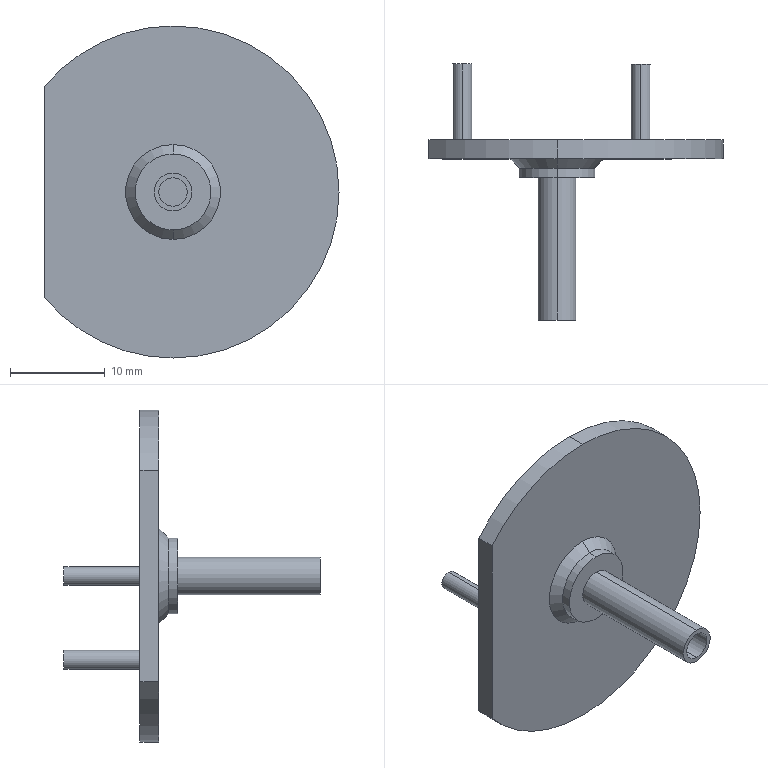Part | SolidWorks | features ICE 6, Chamfer 1, Extrusion 1 | 1 solid | 26 faces | box 31 x 27 x 35 mm | volume 2012 mm3 | cylinder 15 | plane 9 | cone 2 | commonest cylinder face diameters 2 x4 4 x4 35 x3 3 x2 8 x2
STEP:
#1=CARTESIAN_POINT('',(0.,-1.,-2.));
#2=VERTEX_POINT('',#1);
#3=CARTESIAN_POINT('',(0.,-1.,2.));
#4=VERTEX_POINT('',#3);
#5=CARTESIAN_POINT('',(0.,-1.,0.));
#6=DIRECTION('',(0.,1.,0.));
#7=DIRECTION('',(0.,0.,1.));
#8=AXIS2_PLACEMENT_3D('',#5,#6,#7);
#9=CIRCLE('',#8,2.);
#10=EDGE_CURVE('',#2,#4,#9,.T.);
#11=ORIENTED_EDGE('',*,*,#10,.F.);
#12=CARTESIAN_POINT('',(0.,2.,-2.));
#13=VERTEX_POINT('',#12);
#14=CARTESIAN_POINT('',(0.,-1.,-2.));
#15=DIRECTION('',(0.,1.,0.));
#16=VECTOR('',#15,1000.);
#17=LINE('',#14,#16);
#18=EDGE_CURVE('',#2,#13,#17,.T.);
#19=ORIENTED_EDGE('',*,*,#18,.T.);
#20=CARTESIAN_POINT('',(0.,2.,2.));
#21=VERTEX_POINT('',#20);
#22=CARTESIAN_POINT('',(0.,2.,0.));
#23=DIRECTION('',(0.,1.,0.));
#24=DIRECTION('',(0.,0.,1.));
#25=AXIS2_PLACEMENT_3D('',#22,#23,#24);
#26=CIRCLE('',#25,2.);
#27=EDGE_CURVE('',#13,#21,#26,.T.);
#28=ORIENTED_EDGE('',*,*,#27,.T.);
#29=CARTESIAN_POINT('',(0.,-1.,2.));
#30=DIRECTION('',(0.,1.,0.));
#31=VECTOR('',#30,1000.);
#32=LINE('',#29,#31);
#33=EDGE_CURVE('',#4,#21,#32,.T.);
#34=ORIENTED_EDGE('',*,*,#33,.F.);
#35=EDGE_LOOP('',(#11,#19,#28,#34));
#36=FACE_OUTER_BOUND('',#35,.T.);
#37=CARTESIAN_POINT('',(0.,-1.,0.));
#38=DIRECTION('',(0.,1.,0.));
#39=DIRECTION('',(0.,0.,1.));
#40=AXIS2_PLACEMENT_3D('',#37,#38,#39);
#41=CYLINDRICAL_SURFACE('',#40,2.);
#42=ADVANCED_FACE('',(#36),#41,.F.);
#43=CARTESIAN_POINT('',(8.839,10.,-7.839));
#44=VERTEX_POINT('',#43);
#45=CARTESIAN_POINT('',(8.839,10.,-9.839));
#46=VERTEX_POINT('',#45);
#47=CARTESIAN_POINT('',(8.839,10.,-8.839));
#48=DIRECTION('',(0.,1.,0.));
#49=DIRECTION('',(0.,0.,1.));
#50=AXIS2_PLACEMENT_3D('',#47,#48,#49);
#51=CIRCLE('',#50,1.);
#52=EDGE_CURVE('',#44,#46,#51,.T.);
#53=ORIENTED_EDGE('',*,*,#52,.F.);
#54=CARTESIAN_POINT('',(8.839,2.,-7.839));
#55=VERTEX_POINT('',#54);
#56=CARTESIAN_POINT('',(8.839,10.,-7.839));
#57=DIRECTION('',(0.,-1.,0.));
#58=VECTOR('',#57,1000.);
#59=LINE('',#56,#58);
#60=EDGE_CURVE('',#44,#55,#59,.T.);
#61=ORIENTED_EDGE('',*,*,#60,.T.);
#62=CARTESIAN_POINT('',(8.839,2.,-9.839));
#63=VERTEX_POINT('',#62);
#64=CARTESIAN_POINT('',(8.839,2.,-8.839));
#65=DIRECTION('',(0.,1.,0.));
#66=DIRECTION('',(0.,0.,1.));
#67=AXIS2_PLACEMENT_3D('',#64,#65,#66);
#68=CIRCLE('',#67,1.);
#69=EDGE_CURVE('',#55,#63,#68,.T.);
#70=ORIENTED_EDGE('',*,*,#69,.T.);
#71=CARTESIAN_POINT('',(8.839,10.,-9.839));
#72=DIRECTION('',(0.,-1.,0.));
#73=VECTOR('',#72,1000.);
#74=LINE('',#71,#73);
#75=EDGE_CURVE('',#46,#63,#74,.T.);
#76=ORIENTED_EDGE('',*,*,#75,.F.);
#77=EDGE_LOOP('',(#53,#61,#70,#76));
#78=FACE_OUTER_BOUND('',#77,.T.);
#79=CARTESIAN_POINT('',(8.839,10.,-8.839));
#80=DIRECTION('',(0.,-1.,0.));
#81=DIRECTION('',(0.,0.,-1.));
#82=AXIS2_PLACEMENT_3D('',#79,#80,#81);
#83=CYLINDRICAL_SURFACE('',#82,1.);
#84=ADVANCED_FACE('',(#78),#83,.T.);
#85=CARTESIAN_POINT('',(-10.,10.,1.));
#86=VERTEX_POINT('',#85);
#87=CARTESIAN_POINT('',(-10.,10.,-1.));
#88=VERTEX_POINT('',#87);
#89=CARTESIAN_POINT('',(-10.,10.,0.));
#90=DIRECTION('',(0.,1.,0.));
#91=DIRECTION('',(0.,0.,1.));
#92=AXIS2_PLACEMENT_3D('',#89,#90,#91);
#93=CIRCLE('',#92,1.);
#94=EDGE_CURVE('',#86,#88,#93,.T.);
#95=ORIENTED_EDGE('',*,*,#94,.F.);
#96=CARTESIAN_POINT('',(-10.,2.,1.));
#97=VERTEX_POINT('',#96);
#98=CARTESIAN_POINT('',(-10.,10.,1.));
#99=DIRECTION('',(0.,-1.,0.));
#100=VECTOR('',#99,1000.);
#101=LINE('',#98,#100);
#102=EDGE_CURVE('',#86,#97,#101,.T.);
#103=ORIENTED_EDGE('',*,*,#102,.T.);
#104=CARTESIAN_POINT('',(-10.,2.,-1.));
#105=VERTEX_POINT('',#104);
#106=CARTESIAN_POINT('',(-10.,2.,0.));
#107=DIRECTION('',(0.,1.,0.));
#108=DIRECTION('',(0.,0.,1.));
#109=AXIS2_PLACEMENT_3D('',#106,#107,#108);
#110=CIRCLE('',#109,1.);
#111=EDGE_CURVE('',#97,#105,#110,.T.);
#112=ORIENTED_EDGE('',*,*,#111,.T.);
#113=CARTESIAN_POINT('',(-10.,10.,-1.));
#114=DIRECTION('',(0.,-1.,0.));
#115=VECTOR('',#114,1000.);
#116=LINE('',#113,#115);
#117=EDGE_CURVE('',#88,#105,#116,.T.);
#118=ORIENTED_EDGE('',*,*,#117,.F.);
#119=EDGE_LOOP('',(#95,#103,#112,#118));
#120=FACE_OUTER_BOUND('',#119,.T.);
#121=CARTESIAN_POINT('',(-10.,10.,0.));
#122=DIRECTION('',(0.,-1.,0.));
#123=DIRECTION('',(0.,0.,-1.));
#124=AXIS2_PLACEMENT_3D('',#121,#122,#123);
#125=CYLINDRICAL_SURFACE('',#124,1.);
#126=ADVANCED_FACE('',(#120),#125,.T.);
#127=CARTESIAN_POINT('',(0.,-2.,-1.5));
#128=VERTEX_POINT('',#127);
#129=CARTESIAN_POINT('',(0.,-2.,1.5));
#130=VERTEX_POINT('',#129);
#131=CARTESIAN_POINT('',(0.,-2.,0.));
#132=DIRECTION('',(0.,1.,0.));
#133=DIRECTION('',(0.,0.,-1.));
#134=AXIS2_PLACEMENT_3D('',#131,#132,#133);
#135=CIRCLE('',#134,1.5);
#136=EDGE_CURVE('',#128,#130,#135,.T.);
#137=ORIENTED_EDGE('',*,*,#136,.T.);
#138=CARTESIAN_POINT('',(0.,-17.,1.5));
#139=VERTEX_POINT('',#138);
#140=CARTESIAN_POINT('',(0.,2.243,1.5));
#141=DIRECTION('',(0.,-1.,0.));
#142=VECTOR('',#141,1000.);
#143=LINE('',#140,#142);
#144=EDGE_CURVE('',#130,#139,#143,.T.);
#145=ORIENTED_EDGE('',*,*,#144,.T.);
#146=CARTESIAN_POINT('',(0.,-17.,-1.5));
#147=VERTEX_POINT('',#146);
#148=CARTESIAN_POINT('',(0.,-17.,0.));
#149=DIRECTION('',(0.,-1.,0.));
#150=DIRECTION('',(0.,0.,-1.));
#151=AXIS2_PLACEMENT_3D('',#148,#149,#150);
#152=CIRCLE('',#151,1.5);
#153=EDGE_CURVE('',#139,#147,#152,.T.);
#154=ORIENTED_EDGE('',*,*,#153,.T.);
#155=CARTESIAN_POINT('',(0.,2.243,-1.5));
#156=DIRECTION('',(0.,-1.,0.));
#157=VECTOR('',#156,1000.);
#158=LINE('',#155,#157);
#159=EDGE_CURVE('',#128,#147,#158,.T.);
#160=ORIENTED_EDGE('',*,*,#159,.F.);
#161=EDGE_LOOP('',(#137,#145,#154,#160));
#162=FACE_OUTER_BOUND('',#161,.T.);
#163=CARTESIAN_POINT('',(0.,2.243,0.));
#164=DIRECTION('',(0.,-1.,0.));
#165=DIRECTION('',(0.,0.,-1.));
#166=AXIS2_PLACEMENT_3D('',#163,#164,#165);
#167=CYLINDRICAL_SURFACE('',#166,1.5);
#168=ADVANCED_FACE('',(#162),#167,.F.);
#169=CARTESIAN_POINT('',(0.,-17.,-2.));
#170=VERTEX_POINT('',#169);
#171=CARTESIAN_POINT('',(0.,-17.,2.));
#172=VERTEX_POINT('',#171);
#173=CARTESIAN_POINT('',(0.,-17.,0.));
#174=DIRECTION('',(0.,-1.,0.));
#175=DIRECTION('',(0.,0.,-1.));
#176=AXIS2_PLACEMENT_3D('',#173,#174,#175);
#177=CIRCLE('',#176,2.);
#178=EDGE_CURVE('',#170,#172,#177,.T.);
#179=ORIENTED_EDGE('',*,*,#178,.F.);
#180=CARTESIAN_POINT('',(0.,-2.,-2.));
#181=VERTEX_POINT('',#180);
#182=CARTESIAN_POINT('',(0.,-17.,-2.));
#183=DIRECTION('',(0.,1.,0.));
#184=VECTOR('',#183,1000.);
#185=LINE('',#182,#184);
#186=EDGE_CURVE('',#170,#181,#185,.T.);
#187=ORIENTED_EDGE('',*,*,#186,.T.);
#188=CARTESIAN_POINT('',(0.,-2.,2.));
#189=VERTEX_POINT('',#188);
#190=CARTESIAN_POINT('',(0.,-2.,0.));
#191=DIRECTION('',(0.,-1.,0.));
#192=DIRECTION('',(0.,0.,-1.));
#193=AXIS2_PLACEMENT_3D('',#190,#191,#192);
#194=CIRCLE('',#193,2.);
#195=EDGE_CURVE('',#181,#189,#194,.T.);
#196=ORIENTED_EDGE('',*,*,#195,.T.);
#197=CARTESIAN_POINT('',(0.,-17.,2.));
#198=DIRECTION('',(0.,1.,0.));
#199=VECTOR('',#198,1000.);
#200=LINE('',#197,#199);
#201=EDGE_CURVE('',#172,#189,#200,.T.);
#202=ORIENTED_EDGE('',*,*,#201,.F.);
#203=EDGE_LOOP('',(#179,#187,#196,#202));
#204=FACE_OUTER_BOUND('',#203,.T.);
#205=CARTESIAN_POINT('',(0.,-17.,0.));
#206=DIRECTION('',(0.,1.,0.));
#207=DIRECTION('',(0.,0.,1.));
#208=AXIS2_PLACEMENT_3D('',#205,#206,#207);
#209=CYLINDRICAL_SURFACE('',#208,2.);
#210=ADVANCED_FACE('',(#204),#209,.T.);
#211=CARTESIAN_POINT('',(0.,-1.,-4.));
#212=VERTEX_POINT('',#211);
#213=CARTESIAN_POINT('',(0.,-1.,4.));
#214=VERTEX_POINT('',#213);
#215=CARTESIAN_POINT('',(0.,-1.,0.));
#216=DIRECTION('',(0.,-1.,0.));
#217=DIRECTION('',(0.,0.,1.));
#218=AXIS2_PLACEMENT_3D('',#215,#216,#217);
#219=CIRCLE('',#218,4.);
#220=EDGE_CURVE('',#212,#214,#219,.T.);
#221=ORIENTED_EDGE('',*,*,#220,.F.);
#222=CARTESIAN_POINT('',(0.,0.,-5.));
#223=VERTEX_POINT('',#222);
#224=CARTESIAN_POINT('',(0.,-1.,-4.));
#225=DIRECTION('',(0.,0.7071,-0.7071));
#226=VECTOR('',#225,1000.);
#227=LINE('',#224,#226);
#228=EDGE_CURVE('',#212,#223,#227,.T.);
#229=ORIENTED_EDGE('',*,*,#228,.T.);
#230=CARTESIAN_POINT('',(0.,0.,5.));
#231=VERTEX_POINT('',#230);
#232=CARTESIAN_POINT('',(0.,0.,0.));
#233=DIRECTION('',(0.,1.,0.));
#234=DIRECTION('',(0.,0.,1.));
#235=AXIS2_PLACEMENT_3D('',#232,#233,#234);
#236=CIRCLE('',#235,5.);
#237=EDGE_CURVE('',#231,#223,#236,.T.);
#238=ORIENTED_EDGE('',*,*,#237,.F.);
#239=CARTESIAN_POINT('',(0.,-1.,4.));
#240=DIRECTION('',(0.,0.7071,0.7071));
#241=VECTOR('',#240,1000.);
#242=LINE('',#239,#241);
#243=EDGE_CURVE('',#214,#231,#242,.T.);
#244=ORIENTED_EDGE('',*,*,#243,.F.);
#245=EDGE_LOOP('',(#221,#229,#238,#244));
#246=FACE_OUTER_BOUND('',#245,.T.);
#247=CARTESIAN_POINT('',(0.,-1.,0.));
#248=DIRECTION('',(0.,1.,0.));
#249=DIRECTION('',(0.,0.,1.));
#250=AXIS2_PLACEMENT_3D('',#247,#248,#249);
#251=CONICAL_SURFACE('',#250,4.,0.7854);
#252=ADVANCED_FACE('',(#246),#251,.T.);
#253=CARTESIAN_POINT('',(0.,-2.,-4.));
#254=VERTEX_POINT('',#253);
#255=CARTESIAN_POINT('',(0.,-2.,4.));
#256=VERTEX_POINT('',#255);
#257=CARTESIAN_POINT('',(0.,-2.,0.));
#258=DIRECTION('',(0.,-1.,0.));
#259=DIRECTION('',(0.,0.,-1.));
#260=AXIS2_PLACEMENT_3D('',#257,#258,#259);
#261=CIRCLE('',#260,4.);
#262=EDGE_CURVE('',#254,#256,#261,.T.);
#263=ORIENTED_EDGE('',*,*,#262,.F.);
#264=CARTESIAN_POINT('',(0.,-2.,-4.));
#265=DIRECTION('',(0.,1.,0.));
#266=VECTOR('',#265,1000.);
#267=LINE('',#264,#266);
#268=EDGE_CURVE('',#254,#212,#267,.T.);
#269=ORIENTED_EDGE('',*,*,#268,.T.);
#270=ORIENTED_EDGE('',*,*,#220,.T.);
#271=CARTESIAN_POINT('',(0.,-2.,4.));
#272=DIRECTION('',(0.,1.,0.));
#273=VECTOR('',#272,1000.);
#274=LINE('',#271,#273);
#275=EDGE_CURVE('',#256,#214,#274,.T.);
#276=ORIENTED_EDGE('',*,*,#275,.F.);
#277=EDGE_LOOP('',(#263,#269,#270,#276));
#278=FACE_OUTER_BOUND('',#277,.T.);
#279=CARTESIAN_POINT('',(0.,-2.,0.));
#280=DIRECTION('',(0.,1.,0.));
#281=DIRECTION('',(0.,0.,1.));
#282=AXIS2_PLACEMENT_3D('',#279,#280,#281);
#283=CYLINDRICAL_SURFACE('',#282,4.);
#284=ADVANCED_FACE('',(#278),#283,.T.);
#285=CARTESIAN_POINT('',(0.,2.,17.5));
#286=VERTEX_POINT('',#285);
#287=CARTESIAN_POINT('',(0.,2.,-17.5));
#288=VERTEX_POINT('',#287);
#289=CARTESIAN_POINT('',(0.,2.,0.));
#290=DIRECTION('',(0.,1.,0.));
#291=DIRECTION('',(0.,0.,1.));
#292=AXIS2_PLACEMENT_3D('',#289,#290,#291);
#293=CIRCLE('',#292,17.5);
#294=EDGE_CURVE('',#286,#288,#293,.T.);
#295=ORIENTED_EDGE('',*,*,#294,.F.);
#296=CARTESIAN_POINT('',(0.,0.,17.5));
#297=VERTEX_POINT('',#296);
#298=CARTESIAN_POINT('',(0.,2.,17.5));
#299=DIRECTION('',(0.,-1.,0.));
#300=VECTOR('',#299,1000.);
#301=LINE('',#298,#300);
#302=EDGE_CURVE('',#286,#297,#301,.T.);
#303=ORIENTED_EDGE('',*,*,#302,.T.);
#304=CARTESIAN_POINT('',(0.,0.,-17.5));
#305=VERTEX_POINT('',#304);
#306=CARTESIAN_POINT('',(0.,0.,0.));
#307=DIRECTION('',(0.,1.,0.));
#308=DIRECTION('',(0.,0.,1.));
#309=AXIS2_PLACEMENT_3D('',#306,#307,#308);
#310=CIRCLE('',#309,17.5);
#311=EDGE_CURVE('',#297,#305,#310,.T.);
#312=ORIENTED_EDGE('',*,*,#311,.T.);
#313=CARTESIAN_POINT('',(0.,2.,-17.5));
#314=DIRECTION('',(0.,-1.,0.));
#315=VECTOR('',#314,1000.);
#316=LINE('',#313,#315);
#317=EDGE_CURVE('',#288,#305,#316,.T.);
#318=ORIENTED_EDGE('',*,*,#317,.F.);
#319=EDGE_LOOP('',(#295,#303,#312,#318));
#320=FACE_OUTER_BOUND('',#319,.T.);
#321=CARTESIAN_POINT('',(0.,2.,0.));
#322=DIRECTION('',(0.,-1.,0.));
#323=DIRECTION('',(0.,0.,-1.));
#324=AXIS2_PLACEMENT_3D('',#321,#322,#323);
#325=CYLINDRICAL_SURFACE('',#324,17.5);
#326=ADVANCED_FACE('',(#320),#325,.T.);
#327=CARTESIAN_POINT('',(-13.5,2.,-11.136));
#328=VERTEX_POINT('',#327);
#329=CARTESIAN_POINT('',(0.,2.,0.));
#330=DIRECTION('',(0.,1.,0.));
#331=DIRECTION('',(0.,0.,1.));
#332=AXIS2_PLACEMENT_3D('',#329,#330,#331);
#333=CIRCLE('',#332,17.5);
#334=EDGE_CURVE('',#288,#328,#333,.T.);
#335=ORIENTED_EDGE('',*,*,#334,.F.);
#336=ORIENTED_EDGE('',*,*,#317,.T.);
#337=CARTESIAN_POINT('',(-13.5,0.,-11.136));
#338=VERTEX_POINT('',#337);
#339=CARTESIAN_POINT('',(0.,0.,0.));
#340=DIRECTION('',(0.,1.,0.));
#341=DIRECTION('',(0.,0.,1.));
#342=AXIS2_PLACEMENT_3D('',#339,#340,#341);
#343=CIRCLE('',#342,17.5);
#344=EDGE_CURVE('',#305,#338,#343,.T.);
#345=ORIENTED_EDGE('',*,*,#344,.T.);
#346=CARTESIAN_POINT('',(-13.5,2.,-11.136));
#347=DIRECTION('',(0.,1.,0.));
#348=VECTOR('',#347,1000.);
#349=LINE('',#346,#348);
#350=EDGE_CURVE('',#338,#328,#349,.T.);
#351=ORIENTED_EDGE('',*,*,#350,.T.);
#352=EDGE_LOOP('',(#335,#336,#345,#351));
#353=FACE_OUTER_BOUND('',#352,.T.);
#354=CARTESIAN_POINT('',(0.,2.,0.));
#355=DIRECTION('',(0.,-1.,0.));
#356=DIRECTION('',(0.,0.,-1.));
#357=AXIS2_PLACEMENT_3D('',#354,#355,#356);
#358=CYLINDRICAL_SURFACE('',#357,17.5);
#359=ADVANCED_FACE('',(#353),#358,.T.);
#360=ORIENTED_EDGE('',*,*,#302,.F.);
#361=CARTESIAN_POINT('',(-13.5,2.,11.136));
#362=VERTEX_POINT('',#361);
#363=CARTESIAN_POINT('',(0.,2.,0.));
#364=DIRECTION('',(0.,1.,0.));
#365=DIRECTION('',(0.,0.,1.));
#366=AXIS2_PLACEMENT_3D('',#363,#364,#365);
#367=CIRCLE('',#366,17.5);
#368=EDGE_CURVE('',#362,#286,#367,.T.);
#369=ORIENTED_EDGE('',*,*,#368,.F.);
#370=CARTESIAN_POINT('',(-13.5,0.,11.136));
#371=VERTEX_POINT('',#370);
#372=CARTESIAN_POINT('',(-13.5,2.,11.136));
#373=DIRECTION('',(0.,-1.,0.));
#374=VECTOR('',#373,1000.);
#375=LINE('',#372,#374);
#376=EDGE_CURVE('',#362,#371,#375,.T.);
#377=ORIENTED_EDGE('',*,*,#376,.T.);
#378=CARTESIAN_POINT('',(0.,0.,0.));
#379=DIRECTION('',(0.,1.,0.));
#380=DIRECTION('',(0.,0.,1.));
#381=AXIS2_PLACEMENT_3D('',#378,#379,#380);
#382=CIRCLE('',#381,17.5);
#383=EDGE_CURVE('',#371,#297,#382,.T.);
#384=ORIENTED_EDGE('',*,*,#383,.T.);
#385=EDGE_LOOP('',(#360,#369,#377,#384));
#386=FACE_OUTER_BOUND('',#385,.T.);
#387=CARTESIAN_POINT('',(0.,2.,0.));
#388=DIRECTION('',(0.,-1.,0.));
#389=DIRECTION('',(0.,0.,-1.));
#390=AXIS2_PLACEMENT_3D('',#387,#388,#389);
#391=CYLINDRICAL_SURFACE('',#390,17.5);
#392=ADVANCED_FACE('',(#386),#391,.T.);
#393=CARTESIAN_POINT('',(0.,2.,0.));
#394=DIRECTION('',(0.,1.,0.));
#395=DIRECTION('',(0.,0.,1.));
#396=AXIS2_PLACEMENT_3D('',#393,#394,#395);
#397=CIRCLE('',#396,2.);
#398=EDGE_CURVE('',#21,#13,#397,.T.);
#399=ORIENTED_EDGE('',*,*,#398,.F.);
#400=ORIENTED_EDGE('',*,*,#27,.F.);
#401=EDGE_LOOP('',(#399,#400));
#402=FACE_BOUND('',#401,.T.);
#403=CARTESIAN_POINT('',(-13.5,2.,-22.804));
#404=DIRECTION('',(0.,0.,-1.));
#405=VECTOR('',#404,1000.);
#406=LINE('',#403,#405);
#407=EDGE_CURVE('',#362,#328,#406,.T.);
#408=ORIENTED_EDGE('',*,*,#407,.F.);
#409=ORIENTED_EDGE('',*,*,#368,.T.);
#410=ORIENTED_EDGE('',*,*,#294,.T.);
#411=ORIENTED_EDGE('',*,*,#334,.T.);
#412=EDGE_LOOP('',(#408,#409,#410,#411));
#413=FACE_OUTER_BOUND('',#412,.T.);
#414=CARTESIAN_POINT('',(8.839,2.,-8.839));
#415=DIRECTION('',(0.,1.,0.));
#416=DIRECTION('',(0.,0.,1.));
#417=AXIS2_PLACEMENT_3D('',#414,#415,#416);
#418=CIRCLE('',#417,1.);
#419=EDGE_CURVE('',#63,#55,#418,.T.);
#420=ORIENTED_EDGE('',*,*,#419,.F.);
#421=ORIENTED_EDGE('',*,*,#69,.F.);
#422=EDGE_LOOP('',(#420,#421));
#423=FACE_BOUND('',#422,.T.);
#424=CARTESIAN_POINT('',(-10.,2.,0.));
#425=DIRECTION('',(0.,1.,0.));
#426=DIRECTION('',(0.,0.,1.));
#427=AXIS2_PLACEMENT_3D('',#424,#425,#426);
#428=CIRCLE('',#427,1.);
#429=EDGE_CURVE('',#105,#97,#428,.T.);
#430=ORIENTED_EDGE('',*,*,#429,.F.);
#431=ORIENTED_EDGE('',*,*,#111,.F.);
#432=EDGE_LOOP('',(#430,#431));
#433=FACE_BOUND('',#432,.T.);
#434=CARTESIAN_POINT('',(0.,2.,0.));
#435=DIRECTION('',(0.,1.,0.));
#436=DIRECTION('',(0.,0.,1.));
#437=AXIS2_PLACEMENT_3D('',#434,#435,#436);
#438=PLANE('',#437);
#439=ADVANCED_FACE('',(#402,#413,#423,#433),#438,.T.);
#440=ORIENTED_EDGE('',*,*,#237,.T.);
#441=CARTESIAN_POINT('',(0.,0.,0.));
#442=DIRECTION('',(0.,1.,0.));
#443=DIRECTION('',(0.,0.,1.));
#444=AXIS2_PLACEMENT_3D('',#441,#442,#443);
#445=CIRCLE('',#444,5.);
#446=EDGE_CURVE('',#223,#231,#445,.T.);
#447=ORIENTED_EDGE('',*,*,#446,.T.);
#448=EDGE_LOOP('',(#440,#447));
#449=FACE_BOUND('',#448,.T.);
#450=ORIENTED_EDGE('',*,*,#383,.F.);
#451=CARTESIAN_POINT('',(-13.5,0.,0.));
#452=DIRECTION('',(0.,0.,-1.));
#453=VECTOR('',#452,1000.);
#454=LINE('',#451,#453);
#455=EDGE_CURVE('',#371,#338,#454,.T.);
#456=ORIENTED_EDGE('',*,*,#455,.T.);
#457=ORIENTED_EDGE('',*,*,#344,.F.);
#458=ORIENTED_EDGE('',*,*,#311,.F.);
#459=EDGE_LOOP('',(#450,#456,#457,#458));
#460=FACE_OUTER_BOUND('',#459,.T.);
#461=CARTESIAN_POINT('',(0.,0.,0.));
#462=DIRECTION('',(0.,1.,0.));
#463=DIRECTION('',(0.,0.,1.));
#464=AXIS2_PLACEMENT_3D('',#461,#462,#463);
#465=PLANE('',#464);
#466=ADVANCED_FACE('',(#449,#460),#465,.F.);
#467=ORIENTED_EDGE('',*,*,#268,.F.);
#468=CARTESIAN_POINT('',(0.,-2.,0.));
#469=DIRECTION('',(0.,-1.,0.));
#470=DIRECTION('',(0.,0.,-1.));
#471=AXIS2_PLACEMENT_3D('',#468,#469,#470);
#472=CIRCLE('',#471,4.);
#473=EDGE_CURVE('',#256,#254,#472,.T.);
#474=ORIENTED_EDGE('',*,*,#473,.F.);
#475=ORIENTED_EDGE('',*,*,#275,.T.);
#476=CARTESIAN_POINT('',(0.,-1.,0.));
#477=DIRECTION('',(0.,-1.,0.));
#478=DIRECTION('',(0.,0.,1.));
#479=AXIS2_PLACEMENT_3D('',#476,#477,#478);
#480=CIRCLE('',#479,4.);
#481=EDGE_CURVE('',#214,#212,#480,.T.);
#482=ORIENTED_EDGE('',*,*,#481,.T.);
#483=EDGE_LOOP('',(#467,#474,#475,#482));
#484=FACE_OUTER_BOUND('',#483,.T.);
#485=CARTESIAN_POINT('',(0.,-2.,0.));
#486=DIRECTION('',(0.,1.,0.));
#487=DIRECTION('',(0.,0.,1.));
#488=AXIS2_PLACEMENT_3D('',#485,#486,#487);
#489=CYLINDRICAL_SURFACE('',#488,4.);
#490=ADVANCED_FACE('',(#484),#489,.T.);
#491=CARTESIAN_POINT('',(0.,-2.,0.));
#492=DIRECTION('',(0.,-1.,0.));
#493=DIRECTION('',(0.,0.,-1.));
#494=AXIS2_PLACEMENT_3D('',#491,#492,#493);
#495=CIRCLE('',#494,2.);
#496=EDGE_CURVE('',#189,#181,#495,.T.);
#497=ORIENTED_EDGE('',*,*,#496,.F.);
#498=ORIENTED_EDGE('',*,*,#195,.F.);
#499=EDGE_LOOP('',(#497,#498));
#500=FACE_BOUND('',#499,.T.);
#501=ORIENTED_EDGE('',*,*,#473,.T.);
#502=ORIENTED_EDGE('',*,*,#262,.T.);
#503=EDGE_LOOP('',(#501,#502));
#504=FACE_OUTER_BOUND('',#503,.T.);
#505=CARTESIAN_POINT('',(0.,-2.,0.));
#506=DIRECTION('',(0.,-1.,0.));
#507=DIRECTION('',(0.,0.,-1.));
#508=AXIS2_PLACEMENT_3D('',#505,#506,#507);
#509=PLANE('',#508);
#510=ADVANCED_FACE('',(#500,#504),#509,.T.);
#511=ORIENTED_EDGE('',*,*,#228,.F.);
#512=ORIENTED_EDGE('',*,*,#481,.F.);
#513=ORIENTED_EDGE('',*,*,#243,.T.);
#514=ORIENTED_EDGE('',*,*,#446,.F.);
#515=EDGE_LOOP('',(#511,#512,#513,#514));
#516=FACE_OUTER_BOUND('',#515,.T.);
#517=CARTESIAN_POINT('',(0.,-1.,0.));
#518=DIRECTION('',(0.,1.,0.));
#519=DIRECTION('',(0.,0.,1.));
#520=AXIS2_PLACEMENT_3D('',#517,#518,#519);
#521=CONICAL_SURFACE('',#520,4.,0.7854);
#522=ADVANCED_FACE('',(#516),#521,.T.);
#523=ORIENTED_EDGE('',*,*,#186,.F.);
#524=CARTESIAN_POINT('',(0.,-17.,0.));
#525=DIRECTION('',(0.,-1.,0.));
#526=DIRECTION('',(0.,0.,-1.));
#527=AXIS2_PLACEMENT_3D('',#524,#525,#526);
#528=CIRCLE('',#527,2.);
#529=EDGE_CURVE('',#172,#170,#528,.T.);
#530=ORIENTED_EDGE('',*,*,#529,.F.);
#531=ORIENTED_EDGE('',*,*,#201,.T.);
#532=ORIENTED_EDGE('',*,*,#496,.T.);
#533=EDGE_LOOP('',(#523,#530,#531,#532));
#534=FACE_OUTER_BOUND('',#533,.T.);
#535=CARTESIAN_POINT('',(0.,-17.,0.));
#536=DIRECTION('',(0.,1.,0.));
#537=DIRECTION('',(0.,0.,1.));
#538=AXIS2_PLACEMENT_3D('',#535,#536,#537);
#539=CYLINDRICAL_SURFACE('',#538,2.);
#540=ADVANCED_FACE('',(#534),#539,.T.);
#541=CARTESIAN_POINT('',(0.,-17.,0.));
#542=DIRECTION('',(0.,-1.,0.));
#543=DIRECTION('',(0.,0.,-1.));
#544=AXIS2_PLACEMENT_3D('',#541,#542,#543);
#545=CIRCLE('',#544,1.5);
#546=EDGE_CURVE('',#147,#139,#545,.T.);
#547=ORIENTED_EDGE('',*,*,#546,.F.);
#548=ORIENTED_EDGE('',*,*,#153,.F.);
#549=EDGE_LOOP('',(#547,#548));
#550=FACE_BOUND('',#549,.T.);
#551=ORIENTED_EDGE('',*,*,#529,.T.);
#552=ORIENTED_EDGE('',*,*,#178,.T.);
#553=EDGE_LOOP('',(#551,#552));
#554=FACE_OUTER_BOUND('',#553,.T.);
#555=CARTESIAN_POINT('',(0.,-17.,0.));
#556=DIRECTION('',(0.,-1.,0.));
#557=DIRECTION('',(0.,0.,-1.));
#558=AXIS2_PLACEMENT_3D('',#555,#556,#557);
#559=PLANE('',#558);
#560=ADVANCED_FACE('',(#550,#554),#559,.T.);
#561=ORIENTED_EDGE('',*,*,#144,.F.);
#562=CARTESIAN_POINT('',(0.,-2.,0.));
#563=DIRECTION('',(0.,1.,0.));
#564=DIRECTION('',(0.,0.,-1.));
#565=AXIS2_PLACEMENT_3D('',#562,#563,#564);
#566=CIRCLE('',#565,1.5);
#567=EDGE_CURVE('',#130,#128,#566,.T.);
#568=ORIENTED_EDGE('',*,*,#567,.T.);
#569=ORIENTED_EDGE('',*,*,#159,.T.);
#570=ORIENTED_EDGE('',*,*,#546,.T.);
#571=EDGE_LOOP('',(#561,#568,#569,#570));
#572=FACE_OUTER_BOUND('',#571,.T.);
#573=CARTESIAN_POINT('',(0.,2.243,0.));
#574=DIRECTION('',(0.,-1.,0.));
#575=DIRECTION('',(0.,0.,-1.));
#576=AXIS2_PLACEMENT_3D('',#573,#574,#575);
#577=CYLINDRICAL_SURFACE('',#576,1.5);
#578=ADVANCED_FACE('',(#572),#577,.F.);
#579=ORIENTED_EDGE('',*,*,#136,.F.);
#580=ORIENTED_EDGE('',*,*,#567,.F.);
#581=EDGE_LOOP('',(#579,#580));
#582=FACE_OUTER_BOUND('',#581,.T.);
#583=CARTESIAN_POINT('',(0.,-2.,0.));
#584=DIRECTION('',(0.,-1.,0.));
#585=DIRECTION('',(0.,0.,-1.));
#586=AXIS2_PLACEMENT_3D('',#583,#584,#585);
#587=PLANE('',#586);
#588=ADVANCED_FACE('',(#582),#587,.T.);
#589=ORIENTED_EDGE('',*,*,#102,.F.);
#590=CARTESIAN_POINT('',(-10.,10.,0.));
#591=DIRECTION('',(0.,1.,0.));
#592=DIRECTION('',(0.,0.,1.));
#593=AXIS2_PLACEMENT_3D('',#590,#591,#592);
#594=CIRCLE('',#593,1.);
#595=EDGE_CURVE('',#88,#86,#594,.T.);
#596=ORIENTED_EDGE('',*,*,#595,.F.);
#597=ORIENTED_EDGE('',*,*,#117,.T.);
#598=ORIENTED_EDGE('',*,*,#429,.T.);
#599=EDGE_LOOP('',(#589,#596,#597,#598));
#600=FACE_OUTER_BOUND('',#599,.T.);
#601=CARTESIAN_POINT('',(-10.,10.,0.));
#602=DIRECTION('',(0.,-1.,0.));
#603=DIRECTION('',(0.,0.,-1.));
#604=AXIS2_PLACEMENT_3D('',#601,#602,#603);
#605=CYLINDRICAL_SURFACE('',#604,1.);
#606=ADVANCED_FACE('',(#600),#605,.T.);
#607=ORIENTED_EDGE('',*,*,#595,.T.);
#608=ORIENTED_EDGE('',*,*,#94,.T.);
#609=EDGE_LOOP('',(#607,#608));
#610=FACE_OUTER_BOUND('',#609,.T.);
#611=CARTESIAN_POINT('',(-10.,10.,0.));
#612=DIRECTION('',(0.,1.,0.));
#613=DIRECTION('',(0.,0.,1.));
#614=AXIS2_PLACEMENT_3D('',#611,#612,#613);
#615=PLANE('',#614);
#616=ADVANCED_FACE('',(#610),#615,.T.);
#617=ORIENTED_EDGE('',*,*,#60,.F.);
#618=CARTESIAN_POINT('',(8.839,10.,-8.839));
#619=DIRECTION('',(0.,1.,0.));
#620=DIRECTION('',(0.,0.,1.));
#621=AXIS2_PLACEMENT_3D('',#618,#619,#620);
#622=CIRCLE('',#621,1.);
#623=EDGE_CURVE('',#46,#44,#622,.T.);
#624=ORIENTED_EDGE('',*,*,#623,.F.);
#625=ORIENTED_EDGE('',*,*,#75,.T.);
#626=ORIENTED_EDGE('',*,*,#419,.T.);
#627=EDGE_LOOP('',(#617,#624,#625,#626));
#628=FACE_OUTER_BOUND('',#627,.T.);
#629=CARTESIAN_POINT('',(8.839,10.,-8.839));
#630=DIRECTION('',(0.,-1.,0.));
#631=DIRECTION('',(0.,0.,-1.));
#632=AXIS2_PLACEMENT_3D('',#629,#630,#631);
#633=CYLINDRICAL_SURFACE('',#632,1.);
#634=ADVANCED_FACE('',(#628),#633,.T.);
#635=ORIENTED_EDGE('',*,*,#623,.T.);
#636=ORIENTED_EDGE('',*,*,#52,.T.);
#637=EDGE_LOOP('',(#635,#636));
#638=FACE_OUTER_BOUND('',#637,.T.);
#639=CARTESIAN_POINT('',(8.839,10.,-8.839));
#640=DIRECTION('',(0.,1.,0.));
#641=DIRECTION('',(0.,0.,1.));
#642=AXIS2_PLACEMENT_3D('',#639,#640,#641);
#643=PLANE('',#642);
#644=ADVANCED_FACE('',(#638),#643,.T.);
#645=ORIENTED_EDGE('',*,*,#407,.T.);
#646=ORIENTED_EDGE('',*,*,#350,.F.);
#647=ORIENTED_EDGE('',*,*,#455,.F.);
#648=ORIENTED_EDGE('',*,*,#376,.F.);
#649=EDGE_LOOP('',(#645,#646,#647,#648));
#650=FACE_OUTER_BOUND('',#649,.T.);
#651=CARTESIAN_POINT('',(-13.5,-17.,-22.804));
#652=DIRECTION('',(1.,0.,0.));
#653=DIRECTION('',(0.,0.,-1.));
#654=AXIS2_PLACEMENT_3D('',#651,#652,#653);
#655=PLANE('',#654);
#656=ADVANCED_FACE('',(#650),#655,.F.);
#657=ORIENTED_EDGE('',*,*,#18,.F.);
#658=CARTESIAN_POINT('',(0.,-1.,0.));
#659=DIRECTION('',(0.,1.,0.));
#660=DIRECTION('',(0.,0.,1.));
#661=AXIS2_PLACEMENT_3D('',#658,#659,#660);
#662=CIRCLE('',#661,2.);
#663=EDGE_CURVE('',#4,#2,#662,.T.);
#664=ORIENTED_EDGE('',*,*,#663,.F.);
#665=ORIENTED_EDGE('',*,*,#33,.T.);
#666=ORIENTED_EDGE('',*,*,#398,.T.);
#667=EDGE_LOOP('',(#657,#664,#665,#666));
#668=FACE_OUTER_BOUND('',#667,.T.);
#669=CARTESIAN_POINT('',(0.,-1.,0.));
#670=DIRECTION('',(0.,1.,0.));
#671=DIRECTION('',(0.,0.,1.));
#672=AXIS2_PLACEMENT_3D('',#669,#670,#671);
#673=CYLINDRICAL_SURFACE('',#672,2.);
#674=ADVANCED_FACE('',(#668),#673,.F.);
#675=ORIENTED_EDGE('',*,*,#663,.T.);
#676=ORIENTED_EDGE('',*,*,#10,.T.);
#677=EDGE_LOOP('',(#675,#676));
#678=FACE_OUTER_BOUND('',#677,.T.);
#679=CARTESIAN_POINT('',(0.,-1.,0.));
#680=DIRECTION('',(0.,1.,0.));
#681=DIRECTION('',(0.,0.,1.));
#682=AXIS2_PLACEMENT_3D('',#679,#680,#681);
#683=PLANE('',#682);
#684=ADVANCED_FACE('',(#678),#683,.T.);
#685=CLOSED_SHELL('',(#42,#84,#126,#168,#210,#252,#284,#326,#359,#392,#439,#466,#490,#510,#522,#540,#560,#578,#588,#606,#616,#634,#644,#656,#674,#684));
#686=MANIFOLD_SOLID_BREP('',#685);
#687=CARTESIAN_POINT('',(0.,0.,0.));
#688=DIRECTION('',(0.,0.,1.));
#689=DIRECTION('',(1.,0.,0.));
#690=AXIS2_PLACEMENT_3D('',#687,#688,#689);
#691=(LENGTH_UNIT()NAMED_UNIT(*)SI_UNIT(.MILLI.,.METRE.));
#692=UNCERTAINTY_MEASURE_WITH_UNIT(LENGTH_MEASURE(0.00001),#691,'','');
#693=(NAMED_UNIT(*)PLANE_ANGLE_UNIT()SI_UNIT($,.RADIAN.));
#694=(NAMED_UNIT(*)SI_UNIT($,.STERADIAN.)SOLID_ANGLE_UNIT());
#695=(GEOMETRIC_REPRESENTATION_CONTEXT(3)GLOBAL_UNCERTAINTY_ASSIGNED_CONTEXT((#692))GLOBAL_UNIT_ASSIGNED_CONTEXT((#691,#693,#694))REPRESENTATION_CONTEXT('',''));
#696=ADVANCED_BREP_SHAPE_REPRESENTATION('',(#686,#690),#695);